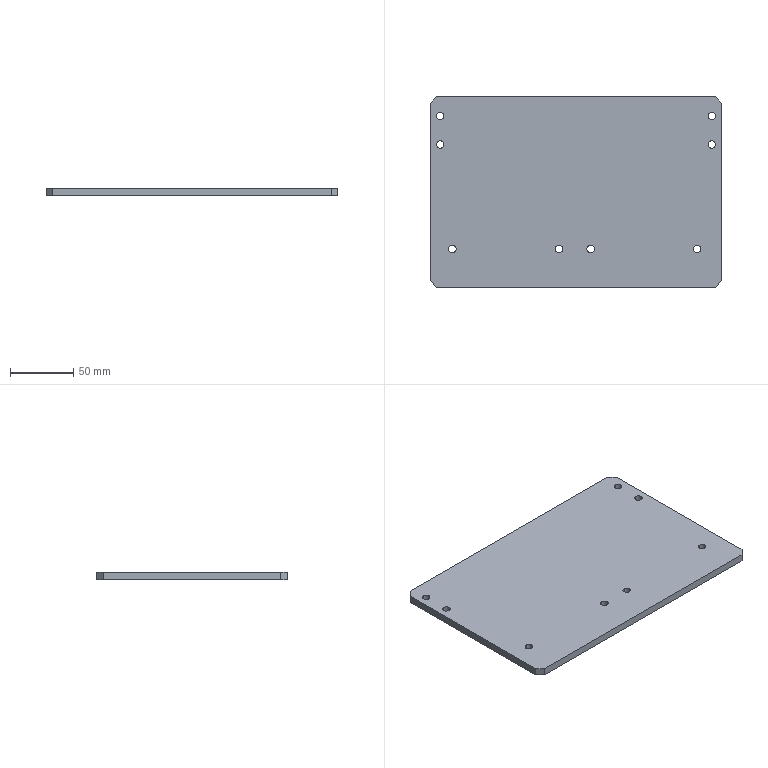Part | STEP file | [02]-8 | 1 solid | 26 faces | box 230 x 150 x 6 mm | volume 205343 mm3 | cylinder 16 | plane 10 | commonest cylinder face diameters 6 x16